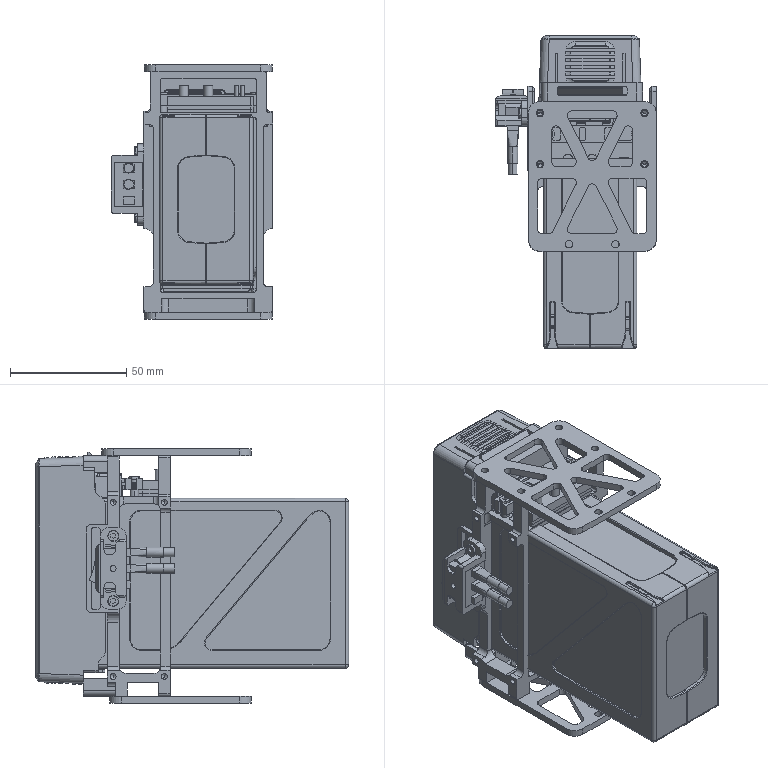Part | SolidWorks | 21 solids | 3763 faces | volume 356333 mm3 | plane 2221 | cylinder 1166 | spline 235 | cone 92 | torus 41 | sphere 8 | commonest cylinder face diameters 1 x213 2 x132 4 x112 3 x111 2.5 x86 0.6 x84